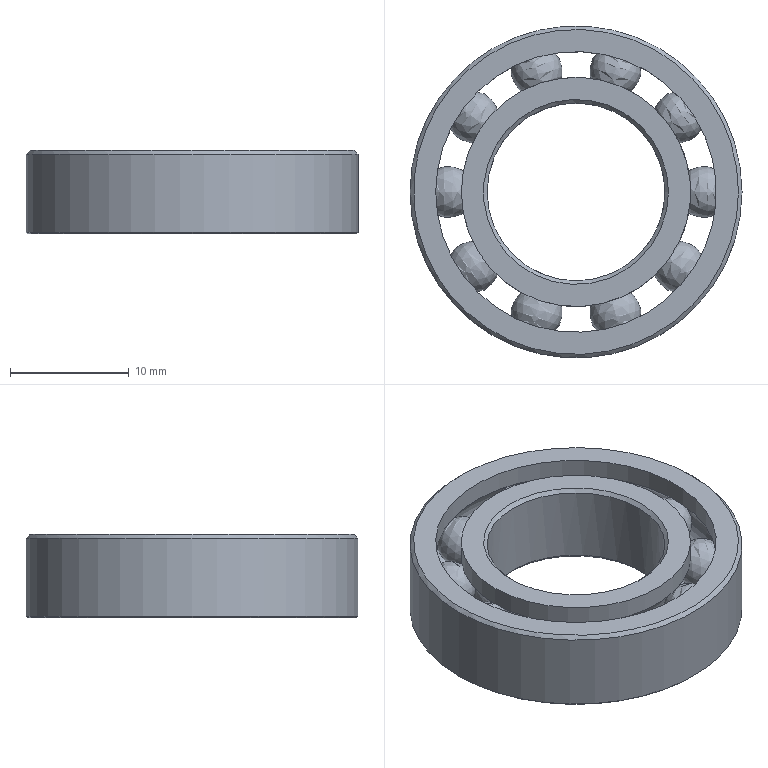Part | NX | features SWP104 15, INSTANCE_SET 9, CHAMFER 3, SKETCH 3, DATUM_CSYS 2, FSET 2, CIRCULAR_PATTERN 1, LINE 1 | 12 solids | 26 faces | box 28 x 28 x 7 mm | volume 2050 mm3 | sphere 10 | cylinder 5 | cone 5 | plane 4 | torus 2 | commonest cylinder face diameters 19.334 x2 15 x1 23.666 x1 28 x1
STEP:
#1=CARTESIAN_POINT('',(6.944,5.045,3.5));
#2=VERTEX_POINT('',#1);
#3=VERTEX_LOOP('',#2);
#4=FACE_BOUND('',#3,.T.);
#5=CARTESIAN_POINT('',(8.697,6.319,3.5));
#6=DIRECTION('',(0.809,0.5878,0.));
#7=DIRECTION('',(0.,0.,1.));
#8=AXIS2_PLACEMENT_3D('',#5,#6,#7);
#9=SPHERICAL_SURFACE('',#8,2.166);
#10=ADVANCED_FACE('',(#4),#9,.T.);
#11=CLOSED_SHELL('',(#10));
#12=MANIFOLD_SOLID_BREP('',#11);
#13=CARTESIAN_POINT('',(-8.584,0.,3.5));
#14=VERTEX_POINT('',#13);
#15=VERTEX_LOOP('',#14);
#16=FACE_BOUND('',#15,.T.);
#17=CARTESIAN_POINT('',(-10.75,0.,3.5));
#18=DIRECTION('',(-1.,0.,0.));
#19=DIRECTION('',(0.,0.,1.));
#20=AXIS2_PLACEMENT_3D('',#17,#18,#19);
#21=SPHERICAL_SURFACE('',#20,2.166);
#22=ADVANCED_FACE('',(#16),#21,.T.);
#23=CLOSED_SHELL('',(#22));
#24=MANIFOLD_SOLID_BREP('',#23);
#25=CARTESIAN_POINT('',(-2.653,8.164,3.5));
#26=VERTEX_POINT('',#25);
#27=VERTEX_LOOP('',#26);
#28=FACE_BOUND('',#27,.T.);
#29=CARTESIAN_POINT('',(-3.322,10.224,3.5));
#30=DIRECTION('',(-0.309,0.9511,0.));
#31=DIRECTION('',(0.,0.,1.));
#32=AXIS2_PLACEMENT_3D('',#29,#30,#31);
#33=SPHERICAL_SURFACE('',#32,2.166);
#34=ADVANCED_FACE('',(#28),#33,.T.);
#35=CLOSED_SHELL('',(#34));
#36=MANIFOLD_SOLID_BREP('',#35);
#37=CARTESIAN_POINT('',(8.584,0.,3.5));
#38=VERTEX_POINT('',#37);
#39=VERTEX_LOOP('',#38);
#40=FACE_BOUND('',#39,.T.);
#41=CARTESIAN_POINT('',(10.75,0.,3.5));
#42=DIRECTION('',(1.,0.,0.));
#43=DIRECTION('',(0.,0.,1.));
#44=AXIS2_PLACEMENT_3D('',#41,#42,#43);
#45=SPHERICAL_SURFACE('',#44,2.166);
#46=ADVANCED_FACE('',(#40),#45,.T.);
#47=CLOSED_SHELL('',(#46));
#48=MANIFOLD_SOLID_BREP('',#47);
#49=CARTESIAN_POINT('',(9.667,0.,1.624));
#50=VERTEX_POINT('',#49);
#51=CARTESIAN_POINT('',(0.,0.,1.624));
#52=DIRECTION('',(0.,0.,1.));
#53=DIRECTION('',(1.,0.,0.));
#54=AXIS2_PLACEMENT_3D('',#51,#52,#53);
#55=CIRCLE('',#54,9.667);
#56=EDGE_CURVE('',#50,#50,#55,.T.);
#57=ORIENTED_EDGE('',*,*,#56,.F.);
#58=EDGE_LOOP('',(#57));
#59=FACE_BOUND('',#58,.T.);
#60=CARTESIAN_POINT('',(-9.667,0.,0.));
#61=VERTEX_POINT('',#60);
#62=CARTESIAN_POINT('',(0.,0.,0.));
#63=DIRECTION('',(0.,0.,-1.));
#64=DIRECTION('',(-1.,0.,0.));
#65=AXIS2_PLACEMENT_3D('',#62,#63,#64);
#66=CIRCLE('',#65,9.667);
#67=EDGE_CURVE('',#61,#61,#66,.T.);
#68=ORIENTED_EDGE('',*,*,#67,.F.);
#69=EDGE_LOOP('',(#68));
#70=FACE_BOUND('',#69,.T.);
#71=CARTESIAN_POINT('',(0.,0.,0.));
#72=DIRECTION('',(0.,0.,-1.));
#73=DIRECTION('',(-1.,0.,0.));
#74=AXIS2_PLACEMENT_3D('',#71,#72,#73);
#75=CYLINDRICAL_SURFACE('',#74,9.667);
#76=ADVANCED_FACE('',(#59,#70),#75,.T.);
#77=CARTESIAN_POINT('',(-7.5,0.,0.3));
#78=VERTEX_POINT('',#77);
#79=CARTESIAN_POINT('',(0.,0.,0.3));
#80=DIRECTION('',(0.,0.,-1.));
#81=DIRECTION('',(-1.,0.,0.));
#82=AXIS2_PLACEMENT_3D('',#79,#80,#81);
#83=CIRCLE('',#82,7.5);
#84=EDGE_CURVE('',#78,#78,#83,.T.);
#85=ORIENTED_EDGE('',*,*,#84,.T.);
#86=EDGE_LOOP('',(#85));
#87=FACE_BOUND('',#86,.T.);
#88=CARTESIAN_POINT('',(7.5,0.,6.7));
#89=VERTEX_POINT('',#88);
#90=CARTESIAN_POINT('',(0.,0.,6.7));
#91=DIRECTION('',(0.,0.,1.));
#92=DIRECTION('',(1.,0.,0.));
#93=AXIS2_PLACEMENT_3D('',#90,#91,#92);
#94=CIRCLE('',#93,7.5);
#95=EDGE_CURVE('',#89,#89,#94,.T.);
#96=ORIENTED_EDGE('',*,*,#95,.T.);
#97=EDGE_LOOP('',(#96));
#98=FACE_BOUND('',#97,.T.);
#99=CARTESIAN_POINT('',(0.,0.,0.));
#100=DIRECTION('',(0.,0.,-1.));
#101=DIRECTION('',(-1.,0.,0.));
#102=AXIS2_PLACEMENT_3D('',#99,#100,#101);
#103=CYLINDRICAL_SURFACE('',#102,7.5);
#104=ADVANCED_FACE('',(#87,#98),#103,.F.);
#105=CARTESIAN_POINT('',(-7.8,0.,0.));
#106=VERTEX_POINT('',#105);
#107=CARTESIAN_POINT('',(0.,0.,0.));
#108=DIRECTION('',(0.,0.,-1.));
#109=DIRECTION('',(-1.,0.,0.));
#110=AXIS2_PLACEMENT_3D('',#107,#108,#109);
#111=CIRCLE('',#110,7.8);
#112=EDGE_CURVE('',#106,#106,#111,.F.);
#113=ORIENTED_EDGE('',*,*,#112,.T.);
#114=EDGE_LOOP('',(#113));
#115=FACE_BOUND('',#114,.T.);
#116=ORIENTED_EDGE('',*,*,#67,.T.);
#117=EDGE_LOOP('',(#116));
#118=FACE_BOUND('',#117,.T.);
#119=CARTESIAN_POINT('',(7.5,0.,0.));
#120=DIRECTION('',(0.,0.,-1.));
#121=DIRECTION('',(-1.,0.,0.));
#122=AXIS2_PLACEMENT_3D('',#119,#120,#121);
#123=PLANE('',#122);
#124=ADVANCED_FACE('',(#115,#118),#123,.T.);
#125=CARTESIAN_POINT('',(-9.667,0.,5.376));
#126=VERTEX_POINT('',#125);
#127=CARTESIAN_POINT('',(0.,0.,5.376));
#128=DIRECTION('',(0.,0.,-1.));
#129=DIRECTION('',(-1.,0.,0.));
#130=AXIS2_PLACEMENT_3D('',#127,#128,#129);
#131=CIRCLE('',#130,9.667);
#132=EDGE_CURVE('',#126,#126,#131,.T.);
#133=ORIENTED_EDGE('',*,*,#132,.F.);
#134=EDGE_LOOP('',(#133));
#135=FACE_BOUND('',#134,.T.);
#136=CARTESIAN_POINT('',(-9.667,0.,7.));
#137=VERTEX_POINT('',#136);
#138=CARTESIAN_POINT('',(0.,0.,7.));
#139=DIRECTION('',(0.,0.,-1.));
#140=DIRECTION('',(-1.,0.,0.));
#141=AXIS2_PLACEMENT_3D('',#138,#139,#140);
#142=CIRCLE('',#141,9.667);
#143=EDGE_CURVE('',#137,#137,#142,.T.);
#144=ORIENTED_EDGE('',*,*,#143,.T.);
#145=EDGE_LOOP('',(#144));
#146=FACE_BOUND('',#145,.T.);
#147=CARTESIAN_POINT('',(0.,0.,0.));
#148=DIRECTION('',(0.,0.,-1.));
#149=DIRECTION('',(-1.,0.,0.));
#150=AXIS2_PLACEMENT_3D('',#147,#148,#149);
#151=CYLINDRICAL_SURFACE('',#150,9.667);
#152=ADVANCED_FACE('',(#135,#146),#151,.T.);
#153=CARTESIAN_POINT('',(7.8,0.,7.));
#154=VERTEX_POINT('',#153);
#155=CARTESIAN_POINT('',(0.,0.,7.));
#156=DIRECTION('',(0.,0.,1.));
#157=DIRECTION('',(1.,0.,0.));
#158=AXIS2_PLACEMENT_3D('',#155,#156,#157);
#159=CIRCLE('',#158,7.8);
#160=EDGE_CURVE('',#154,#154,#159,.F.);
#161=ORIENTED_EDGE('',*,*,#160,.T.);
#162=EDGE_LOOP('',(#161));
#163=FACE_BOUND('',#162,.T.);
#164=ORIENTED_EDGE('',*,*,#143,.F.);
#165=EDGE_LOOP('',(#164));
#166=FACE_BOUND('',#165,.T.);
#167=CARTESIAN_POINT('',(9.667,0.,7.));
#168=DIRECTION('',(0.,0.,1.));
#169=DIRECTION('',(1.,0.,0.));
#170=AXIS2_PLACEMENT_3D('',#167,#168,#169);
#171=PLANE('',#170);
#172=ADVANCED_FACE('',(#163,#166),#171,.T.);
#173=ORIENTED_EDGE('',*,*,#56,.T.);
#174=EDGE_LOOP('',(#173));
#175=FACE_BOUND('',#174,.T.);
#176=ORIENTED_EDGE('',*,*,#132,.T.);
#177=EDGE_LOOP('',(#176));
#178=FACE_BOUND('',#177,.T.);
#179=CARTESIAN_POINT('',(0.,0.,3.5));
#180=DIRECTION('',(0.,0.,-1.));
#181=DIRECTION('',(-1.,0.,0.));
#182=AXIS2_PLACEMENT_3D('',#179,#180,#181);
#183=TOROIDAL_SURFACE('',#182,10.75,2.166);
#184=ADVANCED_FACE('',(#175,#178),#183,.F.);
#185=ORIENTED_EDGE('',*,*,#112,.F.);
#186=EDGE_LOOP('',(#185));
#187=FACE_BOUND('',#186,.T.);
#188=ORIENTED_EDGE('',*,*,#84,.F.);
#189=EDGE_LOOP('',(#188));
#190=FACE_BOUND('',#189,.T.);
#191=CARTESIAN_POINT('',(0.,0.,0.3));
#192=DIRECTION('',(0.,0.,-1.));
#193=DIRECTION('',(-1.,0.,0.));
#194=AXIS2_PLACEMENT_3D('',#191,#192,#193);
#195=CONICAL_SURFACE('',#194,7.5,0.7854);
#196=ADVANCED_FACE('',(#187,#190),#195,.F.);
#197=ORIENTED_EDGE('',*,*,#95,.F.);
#198=EDGE_LOOP('',(#197));
#199=FACE_BOUND('',#198,.T.);
#200=ORIENTED_EDGE('',*,*,#160,.F.);
#201=EDGE_LOOP('',(#200));
#202=FACE_BOUND('',#201,.T.);
#203=CARTESIAN_POINT('',(0.,0.,7.));
#204=DIRECTION('',(0.,0.,1.));
#205=DIRECTION('',(1.,0.,0.));
#206=AXIS2_PLACEMENT_3D('',#203,#204,#205);
#207=CONICAL_SURFACE('',#206,7.8,0.7854);
#208=ADVANCED_FACE('',(#199,#202),#207,.F.);
#209=CLOSED_SHELL('',(#76,#104,#124,#152,#172,#184,#196,#208));
#210=MANIFOLD_SOLID_BREP('',#209);
#211=CARTESIAN_POINT('',(-14.,0.,0.1));
#212=VERTEX_POINT('',#211);
#213=CARTESIAN_POINT('',(0.,0.,0.1));
#214=DIRECTION('',(0.,0.,-1.));
#215=DIRECTION('',(-1.,0.,0.));
#216=AXIS2_PLACEMENT_3D('',#213,#214,#215);
#217=CIRCLE('',#216,14.);
#218=EDGE_CURVE('',#212,#212,#217,.F.);
#219=ORIENTED_EDGE('',*,*,#218,.T.);
#220=EDGE_LOOP('',(#219));
#221=FACE_BOUND('',#220,.T.);
#222=CARTESIAN_POINT('',(14.,0.,6.7));
#223=VERTEX_POINT('',#222);
#224=CARTESIAN_POINT('',(0.,0.,6.7));
#225=DIRECTION('',(0.,0.,1.));
#226=DIRECTION('',(1.,0.,0.));
#227=AXIS2_PLACEMENT_3D('',#224,#225,#226);
#228=CIRCLE('',#227,14.);
#229=EDGE_CURVE('',#223,#223,#228,.F.);
#230=ORIENTED_EDGE('',*,*,#229,.T.);
#231=EDGE_LOOP('',(#230));
#232=FACE_BOUND('',#231,.T.);
#233=CARTESIAN_POINT('',(0.,0.,0.));
#234=DIRECTION('',(0.,0.,-1.));
#235=DIRECTION('',(-1.,0.,0.));
#236=AXIS2_PLACEMENT_3D('',#233,#234,#235);
#237=CYLINDRICAL_SURFACE('',#236,14.);
#238=ADVANCED_FACE('',(#221,#232),#237,.T.);
#239=CARTESIAN_POINT('',(13.7,0.,7.));
#240=VERTEX_POINT('',#239);
#241=CARTESIAN_POINT('',(0.,0.,7.));
#242=DIRECTION('',(0.,0.,1.));
#243=DIRECTION('',(1.,0.,0.));
#244=AXIS2_PLACEMENT_3D('',#241,#242,#243);
#245=CIRCLE('',#244,13.7);
#246=EDGE_CURVE('',#240,#240,#245,.T.);
#247=ORIENTED_EDGE('',*,*,#246,.T.);
#248=EDGE_LOOP('',(#247));
#249=FACE_BOUND('',#248,.T.);
#250=CARTESIAN_POINT('',(-11.833,0.,7.));
#251=VERTEX_POINT('',#250);
#252=CARTESIAN_POINT('',(0.,0.,7.));
#253=DIRECTION('',(0.,0.,-1.));
#254=DIRECTION('',(-1.,0.,0.));
#255=AXIS2_PLACEMENT_3D('',#252,#253,#254);
#256=CIRCLE('',#255,11.833);
#257=EDGE_CURVE('',#251,#251,#256,.T.);
#258=ORIENTED_EDGE('',*,*,#257,.T.);
#259=EDGE_LOOP('',(#258));
#260=FACE_BOUND('',#259,.T.);
#261=CARTESIAN_POINT('',(14.,0.,7.));
#262=DIRECTION('',(0.,0.,1.));
#263=DIRECTION('',(1.,0.,0.));
#264=AXIS2_PLACEMENT_3D('',#261,#262,#263);
#265=PLANE('',#264);
#266=ADVANCED_FACE('',(#249,#260),#265,.T.);
#267=CARTESIAN_POINT('',(-11.833,0.,5.376));
#268=VERTEX_POINT('',#267);
#269=CARTESIAN_POINT('',(0.,0.,5.376));
#270=DIRECTION('',(0.,0.,-1.));
#271=DIRECTION('',(-1.,0.,0.));
#272=AXIS2_PLACEMENT_3D('',#269,#270,#271);
#273=CIRCLE('',#272,11.833);
#274=EDGE_CURVE('',#268,#268,#273,.F.);
#275=ORIENTED_EDGE('',*,*,#274,.F.);
#276=EDGE_LOOP('',(#275));
#277=FACE_BOUND('',#276,.T.);
#278=ORIENTED_EDGE('',*,*,#257,.F.);
#279=EDGE_LOOP('',(#278));
#280=FACE_BOUND('',#279,.T.);
#281=CARTESIAN_POINT('',(0.,0.,0.));
#282=DIRECTION('',(0.,0.,-1.));
#283=DIRECTION('',(-1.,0.,0.));
#284=AXIS2_PLACEMENT_3D('',#281,#282,#283);
#285=CYLINDRICAL_SURFACE('',#284,11.833);
#286=ADVANCED_FACE('',(#277,#280),#285,.F.);
#287=CARTESIAN_POINT('',(-13.9,0.,0.));
#288=VERTEX_POINT('',#287);
#289=CARTESIAN_POINT('',(0.,0.,0.));
#290=DIRECTION('',(0.,0.,-1.));
#291=DIRECTION('',(-1.,0.,0.));
#292=AXIS2_PLACEMENT_3D('',#289,#290,#291);
#293=CIRCLE('',#292,13.9);
#294=EDGE_CURVE('',#288,#288,#293,.T.);
#295=ORIENTED_EDGE('',*,*,#294,.T.);
#296=EDGE_LOOP('',(#295));
#297=FACE_BOUND('',#296,.T.);
#298=CARTESIAN_POINT('',(-12.266,0.,0.));
#299=VERTEX_POINT('',#298);
#300=CARTESIAN_POINT('',(0.,0.,0.));
#301=DIRECTION('',(0.,0.,-1.));
#302=DIRECTION('',(-1.,0.,0.));
#303=AXIS2_PLACEMENT_3D('',#300,#301,#302);
#304=CIRCLE('',#303,12.266);
#305=EDGE_CURVE('',#299,#299,#304,.T.);
#306=ORIENTED_EDGE('',*,*,#305,.F.);
#307=EDGE_LOOP('',(#306));
#308=FACE_BOUND('',#307,.T.);
#309=CARTESIAN_POINT('',(11.833,0.,0.));
#310=DIRECTION('',(0.,0.,-1.));
#311=DIRECTION('',(-1.,0.,0.));
#312=AXIS2_PLACEMENT_3D('',#309,#310,#311);
#313=PLANE('',#312);
#314=ADVANCED_FACE('',(#297,#308),#313,.T.);
#315=CARTESIAN_POINT('',(-11.833,0.,1.624));
#316=VERTEX_POINT('',#315);
#317=CARTESIAN_POINT('',(0.,0.,1.624));
#318=DIRECTION('',(0.,0.,-1.));
#319=DIRECTION('',(-1.,0.,0.));
#320=AXIS2_PLACEMENT_3D('',#317,#318,#319);
#321=CIRCLE('',#320,11.833);
#322=EDGE_CURVE('',#316,#316,#321,.T.);
#323=ORIENTED_EDGE('',*,*,#322,.T.);
#324=EDGE_LOOP('',(#323));
#325=FACE_BOUND('',#324,.T.);
#326=ORIENTED_EDGE('',*,*,#274,.T.);
#327=EDGE_LOOP('',(#326));
#328=FACE_BOUND('',#327,.T.);
#329=CARTESIAN_POINT('',(0.,0.,3.5));
#330=DIRECTION('',(0.,0.,-1.));
#331=DIRECTION('',(-1.,0.,0.));
#332=AXIS2_PLACEMENT_3D('',#329,#330,#331);
#333=TOROIDAL_SURFACE('',#332,10.75,2.166);
#334=ADVANCED_FACE('',(#325,#328),#333,.F.);
#335=ORIENTED_EDGE('',*,*,#322,.F.);
#336=EDGE_LOOP('',(#335));
#337=FACE_BOUND('',#336,.T.);
#338=ORIENTED_EDGE('',*,*,#305,.T.);
#339=EDGE_LOOP('',(#338));
#340=FACE_BOUND('',#339,.T.);
#341=CARTESIAN_POINT('',(0.,0.,0.));
#342=DIRECTION('',(0.,0.,-1.));
#343=DIRECTION('',(-1.,0.,0.));
#344=AXIS2_PLACEMENT_3D('',#341,#342,#343);
#345=CONICAL_SURFACE('',#344,12.266,0.2608);
#346=ADVANCED_FACE('',(#337,#340),#345,.F.);
#347=ORIENTED_EDGE('',*,*,#246,.F.);
#348=EDGE_LOOP('',(#347));
#349=FACE_BOUND('',#348,.T.);
#350=ORIENTED_EDGE('',*,*,#229,.F.);
#351=EDGE_LOOP('',(#350));
#352=FACE_BOUND('',#351,.T.);
#353=CARTESIAN_POINT('',(0.,0.,6.7));
#354=DIRECTION('',(0.,0.,-1.));
#355=DIRECTION('',(-1.,0.,0.));
#356=AXIS2_PLACEMENT_3D('',#353,#354,#355);
#357=CONICAL_SURFACE('',#356,14.,0.7854);
#358=ADVANCED_FACE('',(#349,#352),#357,.T.);
#359=ORIENTED_EDGE('',*,*,#218,.F.);
#360=EDGE_LOOP('',(#359));
#361=FACE_BOUND('',#360,.T.);
#362=ORIENTED_EDGE('',*,*,#294,.F.);
#363=EDGE_LOOP('',(#362));
#364=FACE_BOUND('',#363,.T.);
#365=CARTESIAN_POINT('',(0.,0.,0.));
#366=DIRECTION('',(0.,0.,1.));
#367=DIRECTION('',(1.,0.,0.));
#368=AXIS2_PLACEMENT_3D('',#365,#366,#367);
#369=CONICAL_SURFACE('',#368,13.9,0.7854);
#370=ADVANCED_FACE('',(#361,#364),#369,.T.);
#371=CLOSED_SHELL('',(#238,#266,#286,#314,#334,#346,#358,#370));
#372=MANIFOLD_SOLID_BREP('',#371);
#373=CARTESIAN_POINT('',(-6.944,5.045,3.5));
#374=VERTEX_POINT('',#373);
#375=VERTEX_LOOP('',#374);
#376=FACE_BOUND('',#375,.T.);
#377=CARTESIAN_POINT('',(-8.697,6.319,3.5));
#378=DIRECTION('',(-0.809,0.5878,0.));
#379=DIRECTION('',(0.,0.,1.));
#380=AXIS2_PLACEMENT_3D('',#377,#378,#379);
#381=SPHERICAL_SURFACE('',#380,2.166);
#382=ADVANCED_FACE('',(#376),#381,.T.);
#383=CLOSED_SHELL('',(#382));
#384=MANIFOLD_SOLID_BREP('',#383);
#385=CARTESIAN_POINT('',(6.944,-5.045,3.5));
#386=VERTEX_POINT('',#385);
#387=VERTEX_LOOP('',#386);
#388=FACE_BOUND('',#387,.T.);
#389=CARTESIAN_POINT('',(8.697,-6.319,3.5));
#390=DIRECTION('',(0.809,-0.5878,0.));
#391=DIRECTION('',(0.,0.,1.));
#392=AXIS2_PLACEMENT_3D('',#389,#390,#391);
#393=SPHERICAL_SURFACE('',#392,2.166);
#394=ADVANCED_FACE('',(#388),#393,.T.);
#395=CLOSED_SHELL('',(#394));
#396=MANIFOLD_SOLID_BREP('',#395);
#397=CARTESIAN_POINT('',(-2.653,-8.164,3.5));
#398=VERTEX_POINT('',#397);
#399=VERTEX_LOOP('',#398);
#400=FACE_BOUND('',#399,.T.);
#401=CARTESIAN_POINT('',(-3.322,-10.224,3.5));
#402=DIRECTION('',(-0.309,-0.9511,0.));
#403=DIRECTION('',(0.,0.,1.));
#404=AXIS2_PLACEMENT_3D('',#401,#402,#403);
#405=SPHERICAL_SURFACE('',#404,2.166);
#406=ADVANCED_FACE('',(#400),#405,.T.);
#407=CLOSED_SHELL('',(#406));
#408=MANIFOLD_SOLID_BREP('',#407);
#409=CARTESIAN_POINT('',(-6.944,-5.045,3.5));
#410=VERTEX_POINT('',#409);
#411=VERTEX_LOOP('',#410);
#412=FACE_BOUND('',#411,.T.);
#413=CARTESIAN_POINT('',(-8.697,-6.319,3.5));
#414=DIRECTION('',(-0.809,-0.5878,0.));
#415=DIRECTION('',(0.,0.,1.));
#416=AXIS2_PLACEMENT_3D('',#413,#414,#415);
#417=SPHERICAL_SURFACE('',#416,2.166);
#418=ADVANCED_FACE('',(#412),#417,.T.);
#419=CLOSED_SHELL('',(#418));
#420=MANIFOLD_SOLID_BREP('',#419);
#421=CARTESIAN_POINT('',(2.653,-8.164,3.5));
#422=VERTEX_POINT('',#421);
#423=VERTEX_LOOP('',#422);
#424=FACE_BOUND('',#423,.T.);
#425=CARTESIAN_POINT('',(3.322,-10.224,3.5));
#426=DIRECTION('',(0.309,-0.9511,0.));
#427=DIRECTION('',(0.,0.,1.));
#428=AXIS2_PLACEMENT_3D('',#425,#426,#427);
#429=SPHERICAL_SURFACE('',#428,2.166);
#430=ADVANCED_FACE('',(#424),#429,.T.);
#431=CLOSED_SHELL('',(#430));
#432=MANIFOLD_SOLID_BREP('',#431);
#433=CARTESIAN_POINT('',(2.653,8.164,3.5));
#434=VERTEX_POINT('',#433);
#435=VERTEX_LOOP('',#434);
#436=FACE_BOUND('',#435,.T.);
#437=CARTESIAN_POINT('',(3.322,10.224,3.5));
#438=DIRECTION('',(0.309,0.9511,0.));
#439=DIRECTION('',(0.,0.,1.));
#440=AXIS2_PLACEMENT_3D('',#437,#438,#439);
#441=SPHERICAL_SURFACE('',#440,2.166);
#442=ADVANCED_FACE('',(#436),#441,.T.);
#443=CLOSED_SHELL('',(#442));
#444=MANIFOLD_SOLID_BREP('',#443);
#445=(LENGTH_UNIT()NAMED_UNIT(*)SI_UNIT(.MILLI.,.METRE.));
#446=UNCERTAINTY_MEASURE_WITH_UNIT(LENGTH_MEASURE(0.00001),#445,'','');
#447=(NAMED_UNIT(*)PLANE_ANGLE_UNIT()SI_UNIT($,.RADIAN.));
#448=(NAMED_UNIT(*)SI_UNIT($,.STERADIAN.)SOLID_ANGLE_UNIT());
#449=(GEOMETRIC_REPRESENTATION_CONTEXT(3)GLOBAL_UNCERTAINTY_ASSIGNED_CONTEXT((#446))GLOBAL_UNIT_ASSIGNED_CONTEXT((#445,#447,#448))REPRESENTATION_CONTEXT('',''));
#450=ADVANCED_BREP_SHAPE_REPRESENTATION('',(#12,#24,#36,#48,#210,#372,#384,#396,#408,#420,#432,#444),#449);